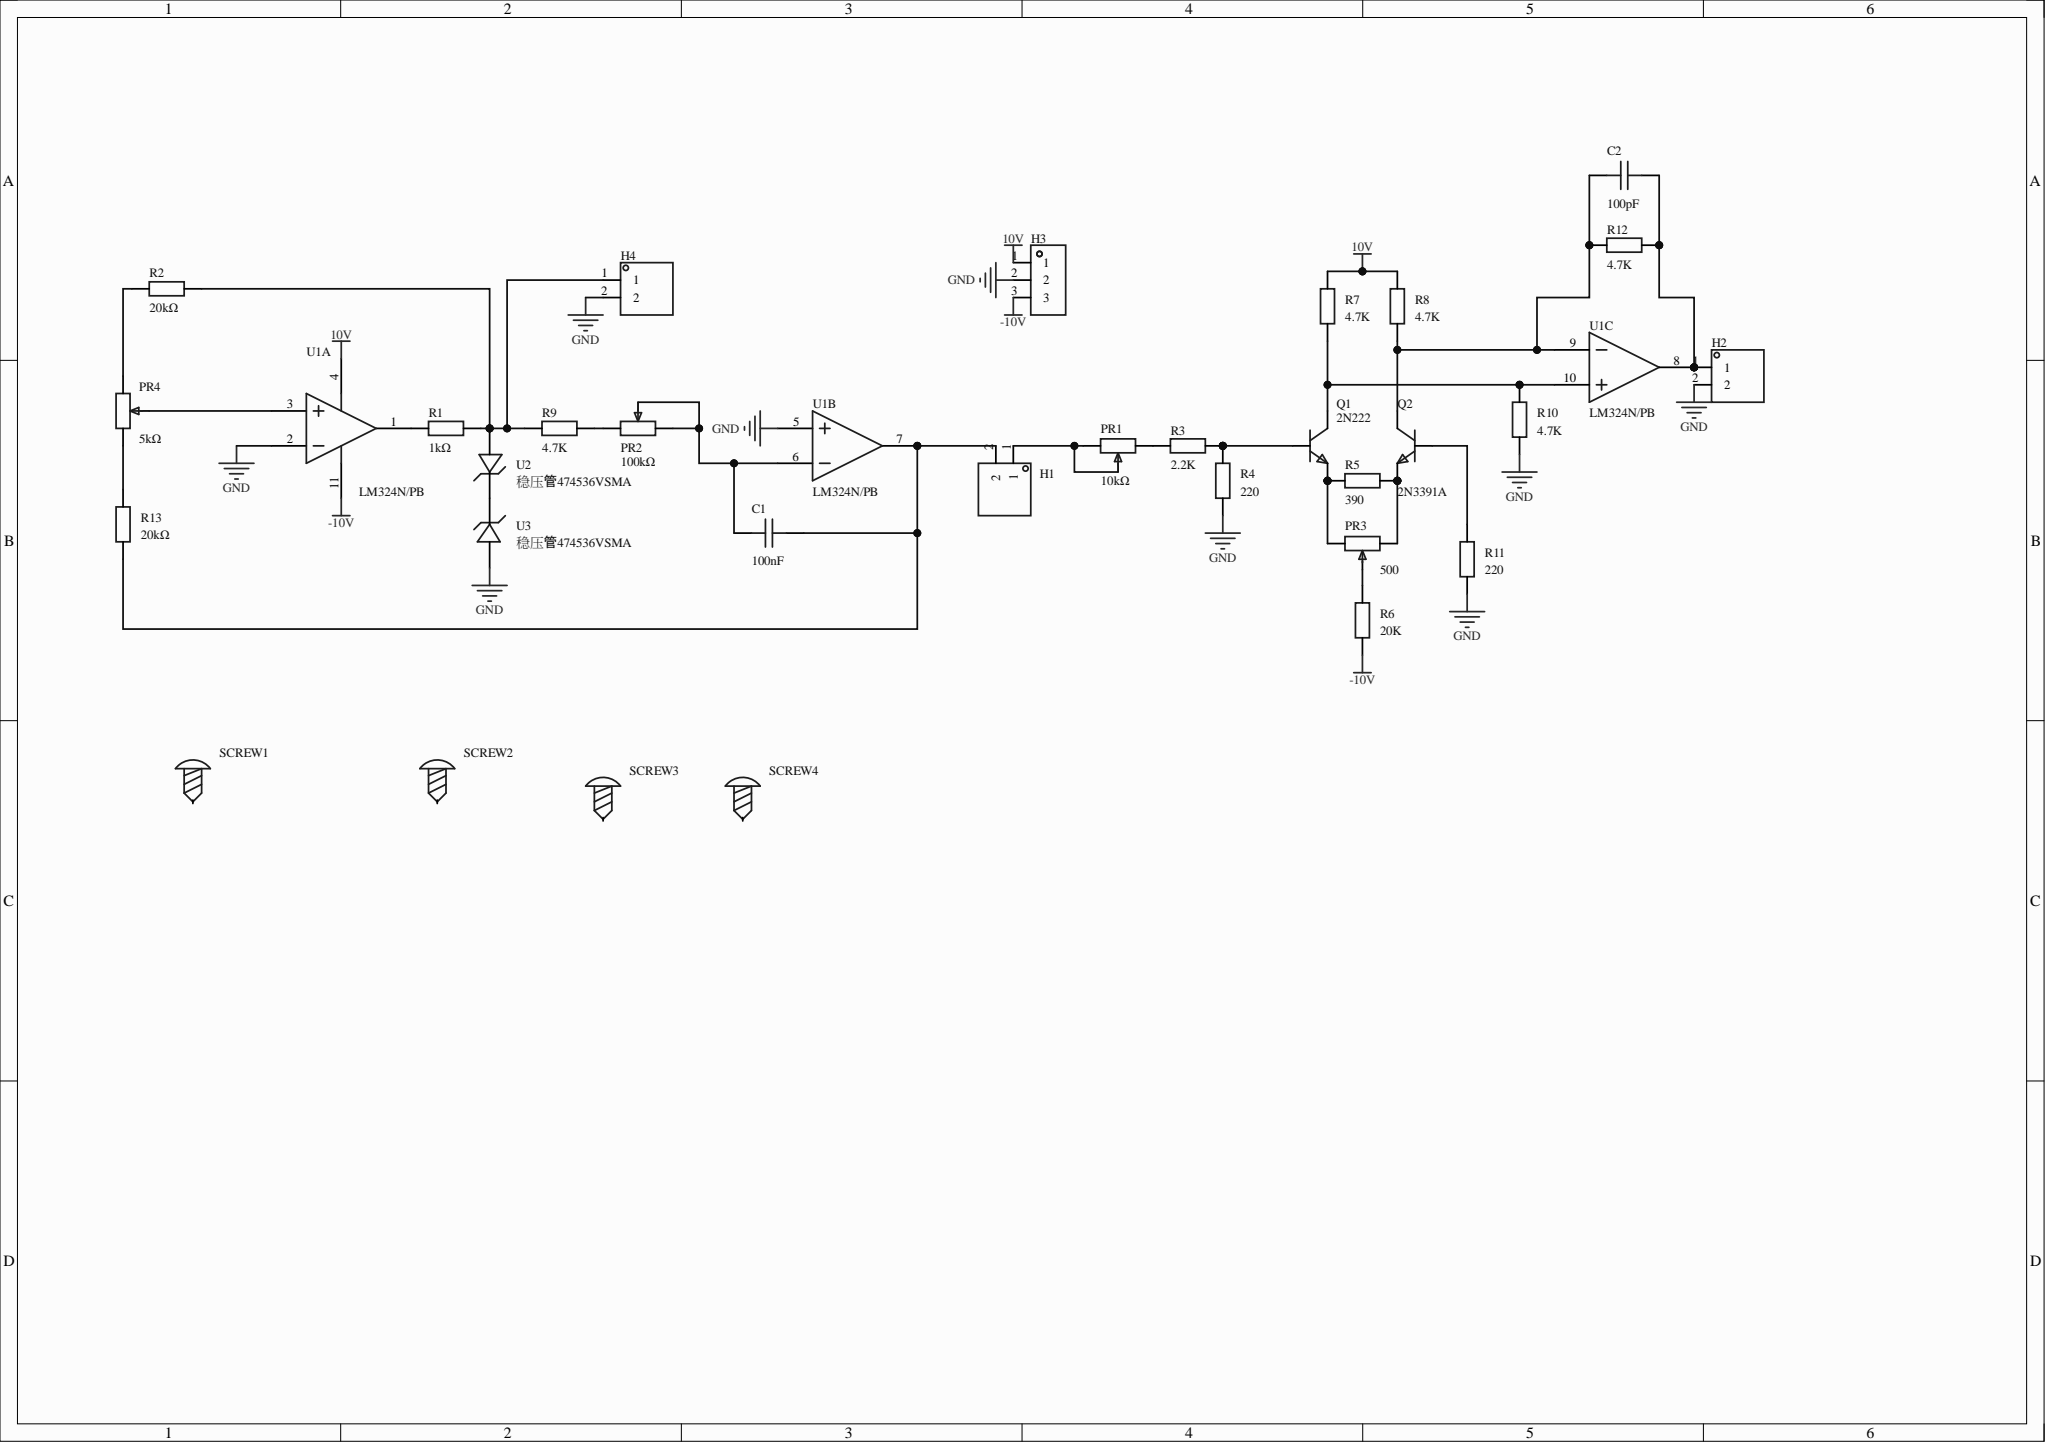Circuit board | Altium Designer | 32 parts | 22 nets
Bill of materials:
Comment,Description,Designator,Footprint,LibRef,Quantity
"100nF","","C1","C0603","CAP_0603","1"
"100pF","","C2","C0603","CAP_0603","1"
"","","H1, H2, H4","HDR-TH_2P-P2.54-V-M-1","HDR-M_2.54_1x2P","3"
"","","H3","HDR-TH_3P-P2.54-V-M","HDR-M_2.54_1x3P","1"
"10kΩ","","PR1","R_3296","R_3296","1"
"100kΩ","","PR2","R_3296","R_3296","1"
"500","","PR3","R_3296","R_3296","1"
"5kΩ","","PR4","R_3296","R_3296","1"
"2N222","晶体管类型:NPN;集电极电流(Ic):800mA;集射极击穿电压(Vceo):50V;功率(Pd):500mW;直流电流增益(hFE@Ic,Vce):30@0.1mA,10V;","Q1","SMD_3-L3.0-W2.5_JANTXV2N2222AUB","JANTX2N2222AUB","1"
"2N3391A","晶体管类型:NPN;集电极电流(Ic):500mA;集射极击穿电压(Vceo):25V;耗散功率(Pd):625mW;直流电流增益(hFE):250@2mA,4.5V;","Q2","TO-92-3_L4.9-W3.7-P1.27-L","2N3391A","1"
"1kΩ","","R1","R0603","Res_0603","1"
"20kΩ","","R2, R13","R0603","Res_0603","2"
"2.2K","","R3","R0603","Res_0603","1"
"220","","R4, R11","R0603","Res_0603","2"
"390","","R5","R0603","Res_0603","1"
"20K","","R6","R0603","Res_0603","1"
"4.7K","","R7, R8, R9, R10, R12","R0603","Res_0603","5"
"","","SCREW1, SCREW2, SCREW3, SCREW4","M2螺丝","M2螺丝","4"
"LM324N/PB","放大器数:四路;增益带宽积(GBP):1MHz;输入偏置电流(Ib):45nA;","U1","PDIP-14_L19.2-W6.6-P2.54-LS7.6-BL","LM324N/PB","1"
"稳压管474536VSMA","","U2, U3","LL-41_L5.0-W2.5-RD","稳压管474536VSMA","2"
Netlist (Protel format):
[
C1
C0603
100nF



]
[
C2
C0603
100pF



]
[
H1
HDR-TH_2P-P2.54-V-M-1




]
[
H2
HDR-TH_2P-P2.54-V-M-1




]
[
H3
HDR-TH_3P-P2.54-V-M




]
[
H4
HDR-TH_2P-P2.54-V-M-1




]
[
PR1
R_3296
10kΩ



]
[
PR2
R_3296
100kΩ



]
[
PR3
R_3296
500



]
[
PR4
R_3296
5kΩ



]
[
Q1
SMD_3-L3.0-W2.5_JANTXV2N2222AUB
2N222



]
[
Q2
TO-92-3_L4.9-W3.7-P1.27-L
2N3391A



]
[
R1
R0603
1kΩ



]
[
R2
R0603
20kΩ



]
[
R3
R0603
2.2K



]
[
R4
R0603
220



]
[
R5
R0603
390



]
[
R6
R0603
20K



]
[
R7
R0603
4.7K



]
[
R8
R0603
4.7K



]
[
R9
R0603
4.7K



]
[
R10
R0603
4.7K



]
[
R11
R0603
220



]
[
R12
R0603
4.7K



]
[
R13
R0603
20kΩ



]
[
SCREW1
M2螺丝




]
[
SCREW2
M2螺丝




]
[
SCREW3
M2螺丝




]
[
SCREW4
M2螺丝




]
[
U1
PDIP-14_L19.2-W6.6-P2.54-LS7.6-BL
LM324N/PB



]
[
U2
LL-41_L5.0-W2.5-RD
稳压管474536VSMA



]
[
U3
LL-41_L5.0-W2.5-RD
稳压管474536VSMA



]
(
NetU2_1
U2-1
U3-1
)
(
NetR1_2
R1-2
U1-1
)
(
NetQ2_3
Q2-3
R11-2
)
(
NetQ1_3
Q1-3
R3-2
R4-2
)
(
NetQ1_1
Q1-1
R7-1
R10-2
U1-10
)
(
NetPR4_3
PR4-3
R2-2
)
(
NetPR4_2
PR4-2
U1-3
)
(
NetPR4_1
PR4-1
R13-1
)
(
NetPR3_3
PR3-3
Q2-1
R5-2
)
(
NetPR3_2
PR3-2
R6-2
)
(
NetPR3_1
PR3-1
Q1-2
R5-1
)
(
NetPR2_3
PR2-3
R9-2
)
(
NetPR1_3
PR1-3
R3-1
)
(
NetH4_1
H4-1
R1-1
R2-1
R9-1
U2-2
)
(
NetH1_1
H1-1
PR1-1
PR1-2
)
(
NetC2_2
C2-2
H2-1
R12-1
U1-8
)
(
NetC2_1
C2-1
Q2-2
R8-1
R12-2
U1-9
)
(
NetC1_2
C1-2
PR2-1
PR2-2
U1-6
)
(
NetC1_1
C1-1
H1-2
R13-2
U1-7
)
(
GND
H2-2
H3-2
H4-2
R4-1
R10-1
R11-1
U1-2
U1-5
U3-2
)
(
-10V
H3-3
R6-1
U1-11
)
(
10V
H3-1
R7-2
R8-2
U1-4
)